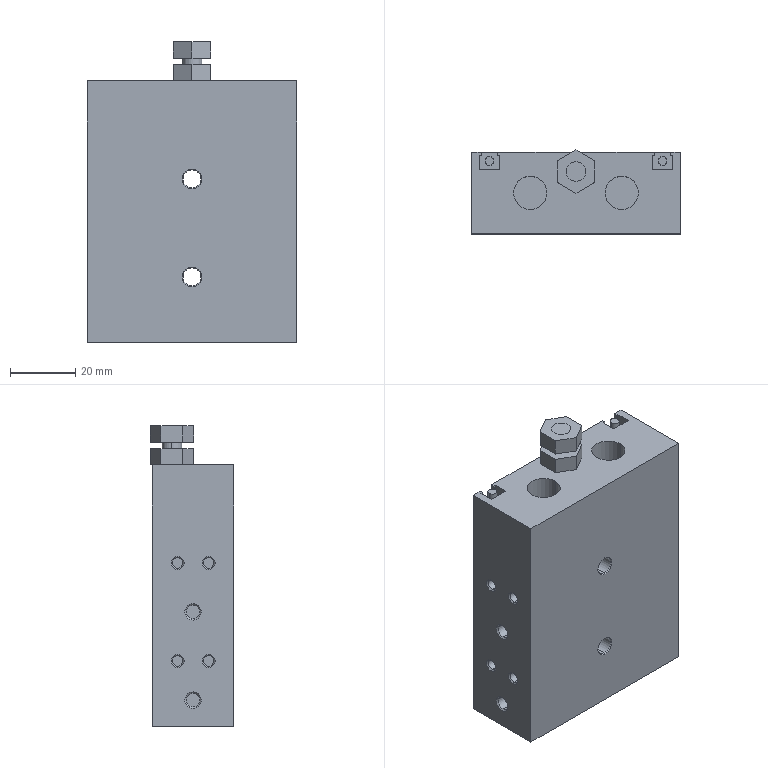Part | STEP file | A_CXSM20-10-Z73 | 1 solid | 147 faces | box 64 x 25.64 x 92 mm | volume 121716 mm3 | plane 75 | cylinder 44 | cone 28 | commonest cylinder face diameters 3.24 x16 4.13 x8 2.7 x4 5.5 x4 6 x4 9.5 x4